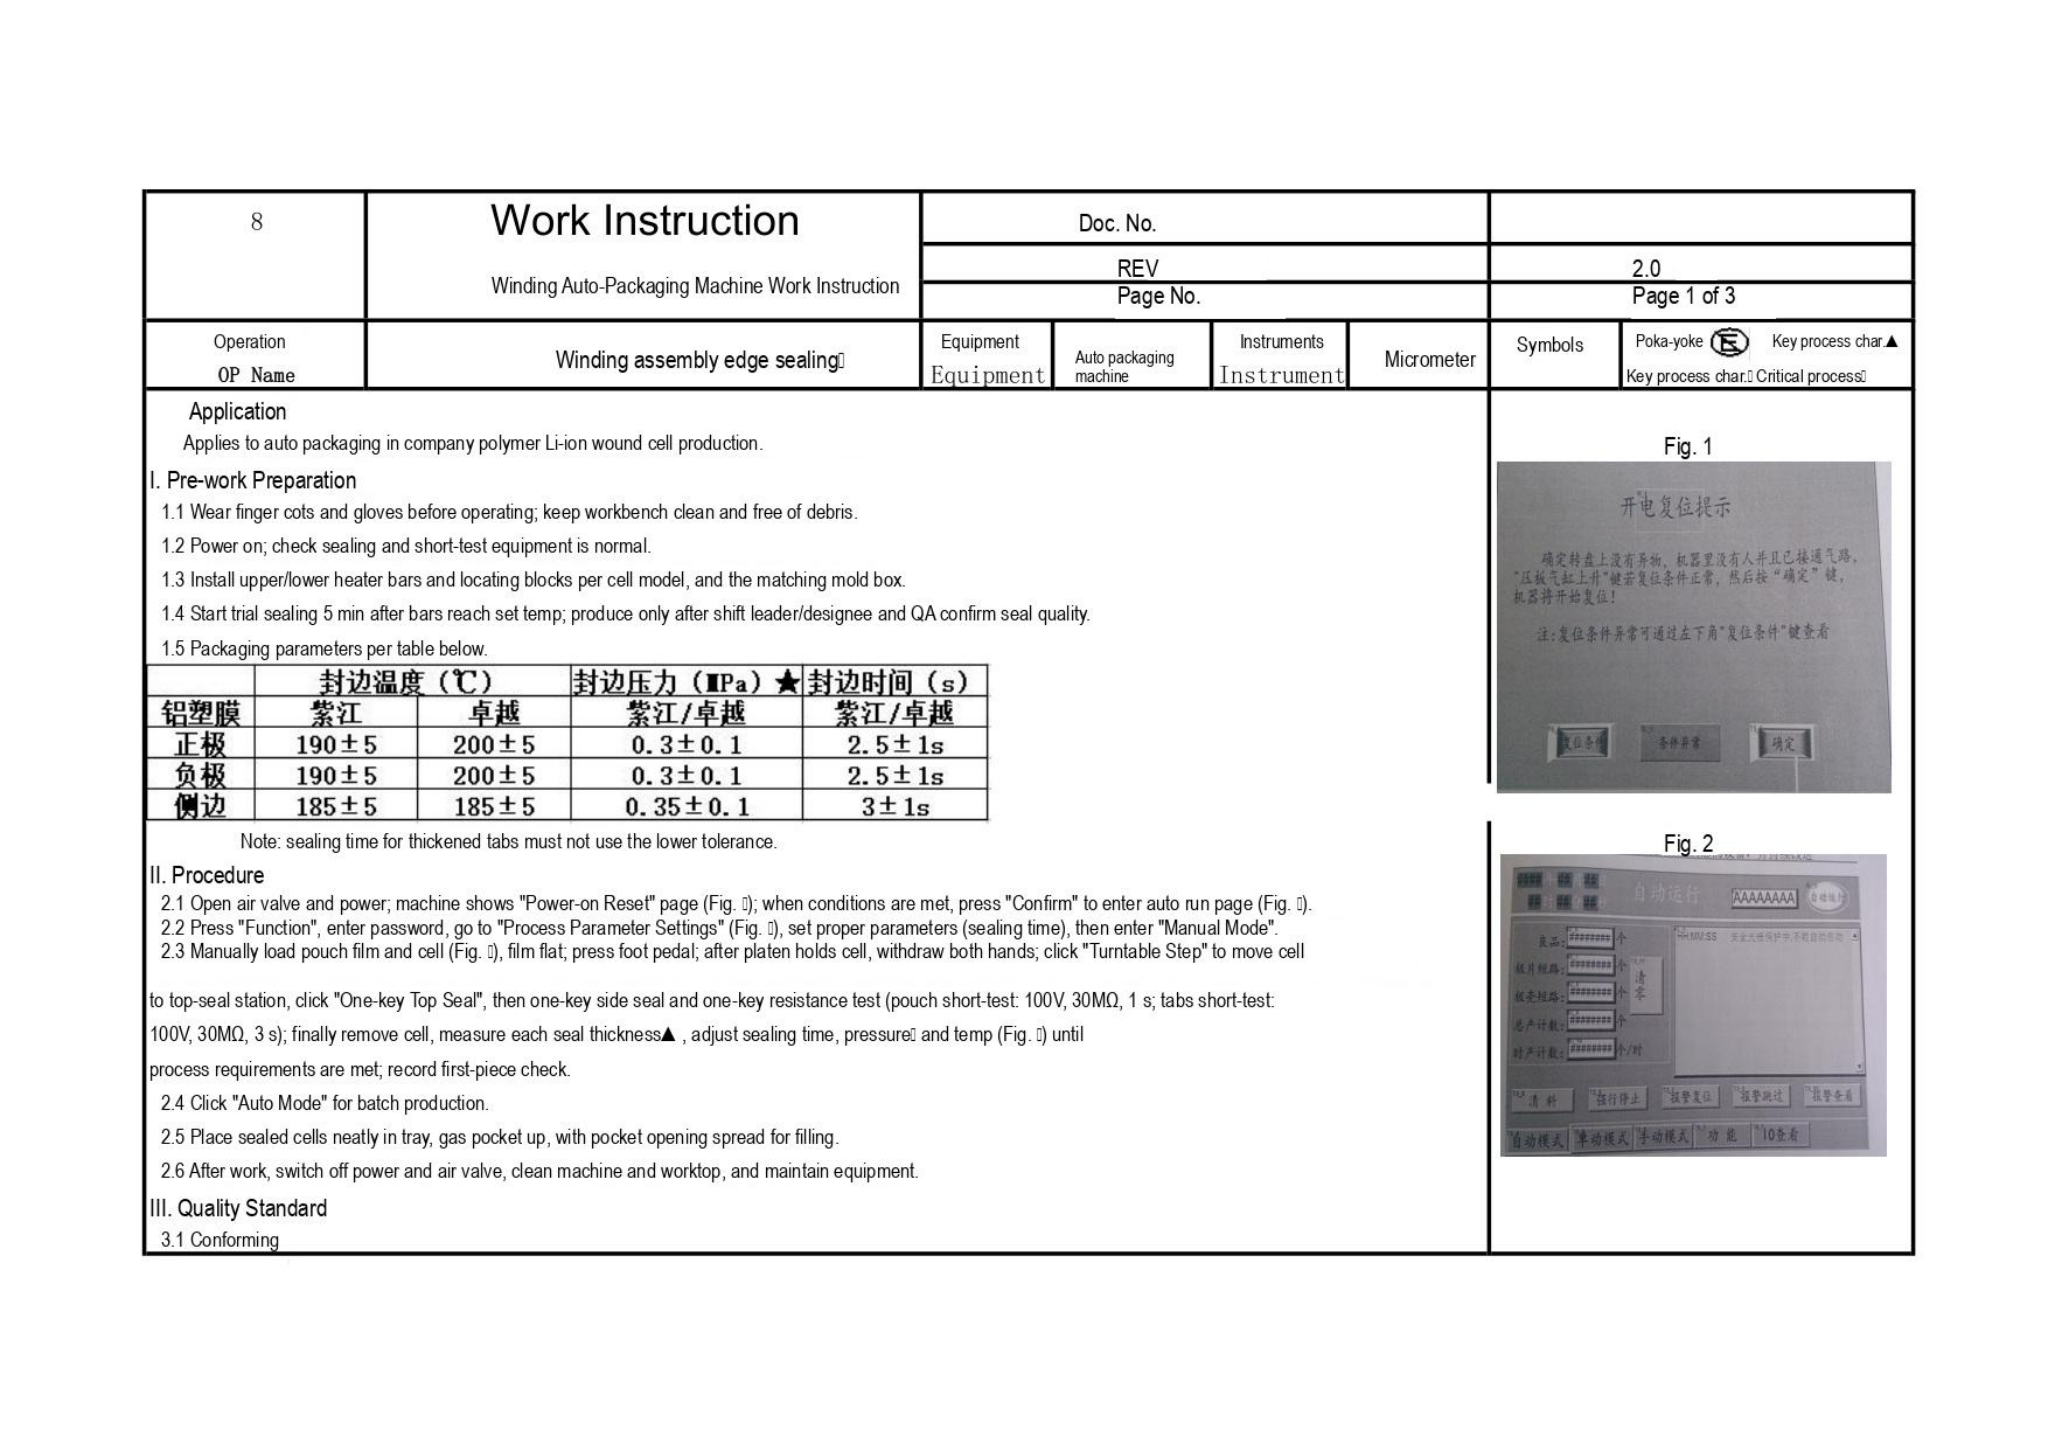8

# Work Instruction

Winding Auto-Packaging Machine Work Instruction

| Doc. No. | |
|---|---|
| REV | 2.0 |
| Page No. | Page 1 of 3 |

| Operation<br>OP Name | Winding assembly edge sealing | Equipment<br>Equipment | Auto packaging machine | Instruments<br>Instrument | Micrometer | Symbols | Poka-yoke Key process char.▲<br>Key process char. Critical process |
|---|---|---|---|---|---|---|---|

Application

Applies to auto packaging in company polymer Li-ion wound cell production.

I. Pre-work Preparation

1.1 Wear finger cots and gloves before operating; keep workbench clean and free of debris.

1.2 Power on; check sealing and short-test equipment is normal.

1.3 Install upper/lower heater bars and locating blocks per cell model, and the matching mold box.

1.4 Start trial sealing 5 min after bars reach set temp; produce only after shift leader/designee and QA confirm seal quality.

1.5 Packaging parameters per table below.

| | 封边温度（℃） | | 封边压力（MPa）★ | 封边时间（s） |
|---|---|---|---|---|
| 铝塑膜 | 紫江 | 卓越 | 紫江/卓越 | 紫江/卓越 |
| 正极 | 190±5 | 200±5 | 0.3±0.1 | 2.5±1s |
| 负极 | 190±5 | 200±5 | 0.3±0.1 | 2.5±1s |
| 侧边 | 185±5 | 185±5 | 0.35±0.1 | 3±1s |

Note: sealing time for thickened tabs must not use the lower tolerance.

II. Procedure

2.1 Open air valve and power; machine shows "Power-on Reset" page (Fig. ); when conditions are met, press "Confirm" to enter auto run page (Fig. ).

2.2 Press "Function", enter password, go to "Process Parameter Settings" (Fig. ), set proper parameters (sealing time), then enter "Manual Mode".

2.3 Manually load pouch film and cell (Fig. ), film flat; press foot pedal; after platen holds cell, withdraw both hands; click "Turntable Step" to move cell

to top-seal station, click "One-key Top Seal", then one-key side seal and one-key resistance test (pouch short-test: 100V, 30MΩ, 1 s; tabs short-test: 100V, 30MΩ, 3 s); finally remove cell, measure each seal thickness▲ , adjust sealing time, pressure and temp (Fig. ) until

process requirements are met; record first-piece check.

2.4 Click "Auto Mode" for batch production.

2.5 Place sealed cells neatly in tray, gas pocket up, with pocket opening spread for filling.

2.6 After work, switch off power and air valve, clean machine and worktop, and maintain equipment.

III. Quality Standard

3.1 Conforming

Fig. 1

开电复位提示

确定转盘上没有异物，机器里没有人并且已接通气路，"压板气缸上升"键若复位条件正常，然后按"确定"键，机器将开始复位！

注：复位条件异常可通过左下角"复位条件"键查看

复位条件 条件异常 确定

Fig. 2

自动运行 AAAAAAAA

良品 个

总产计数 个

时产计数 个/时

清零

HH:MM:SS

清 料 运行停止 报警复位 报警跳过 报警查看

自动模式 单动模式 手动模式 功 能 IO查看
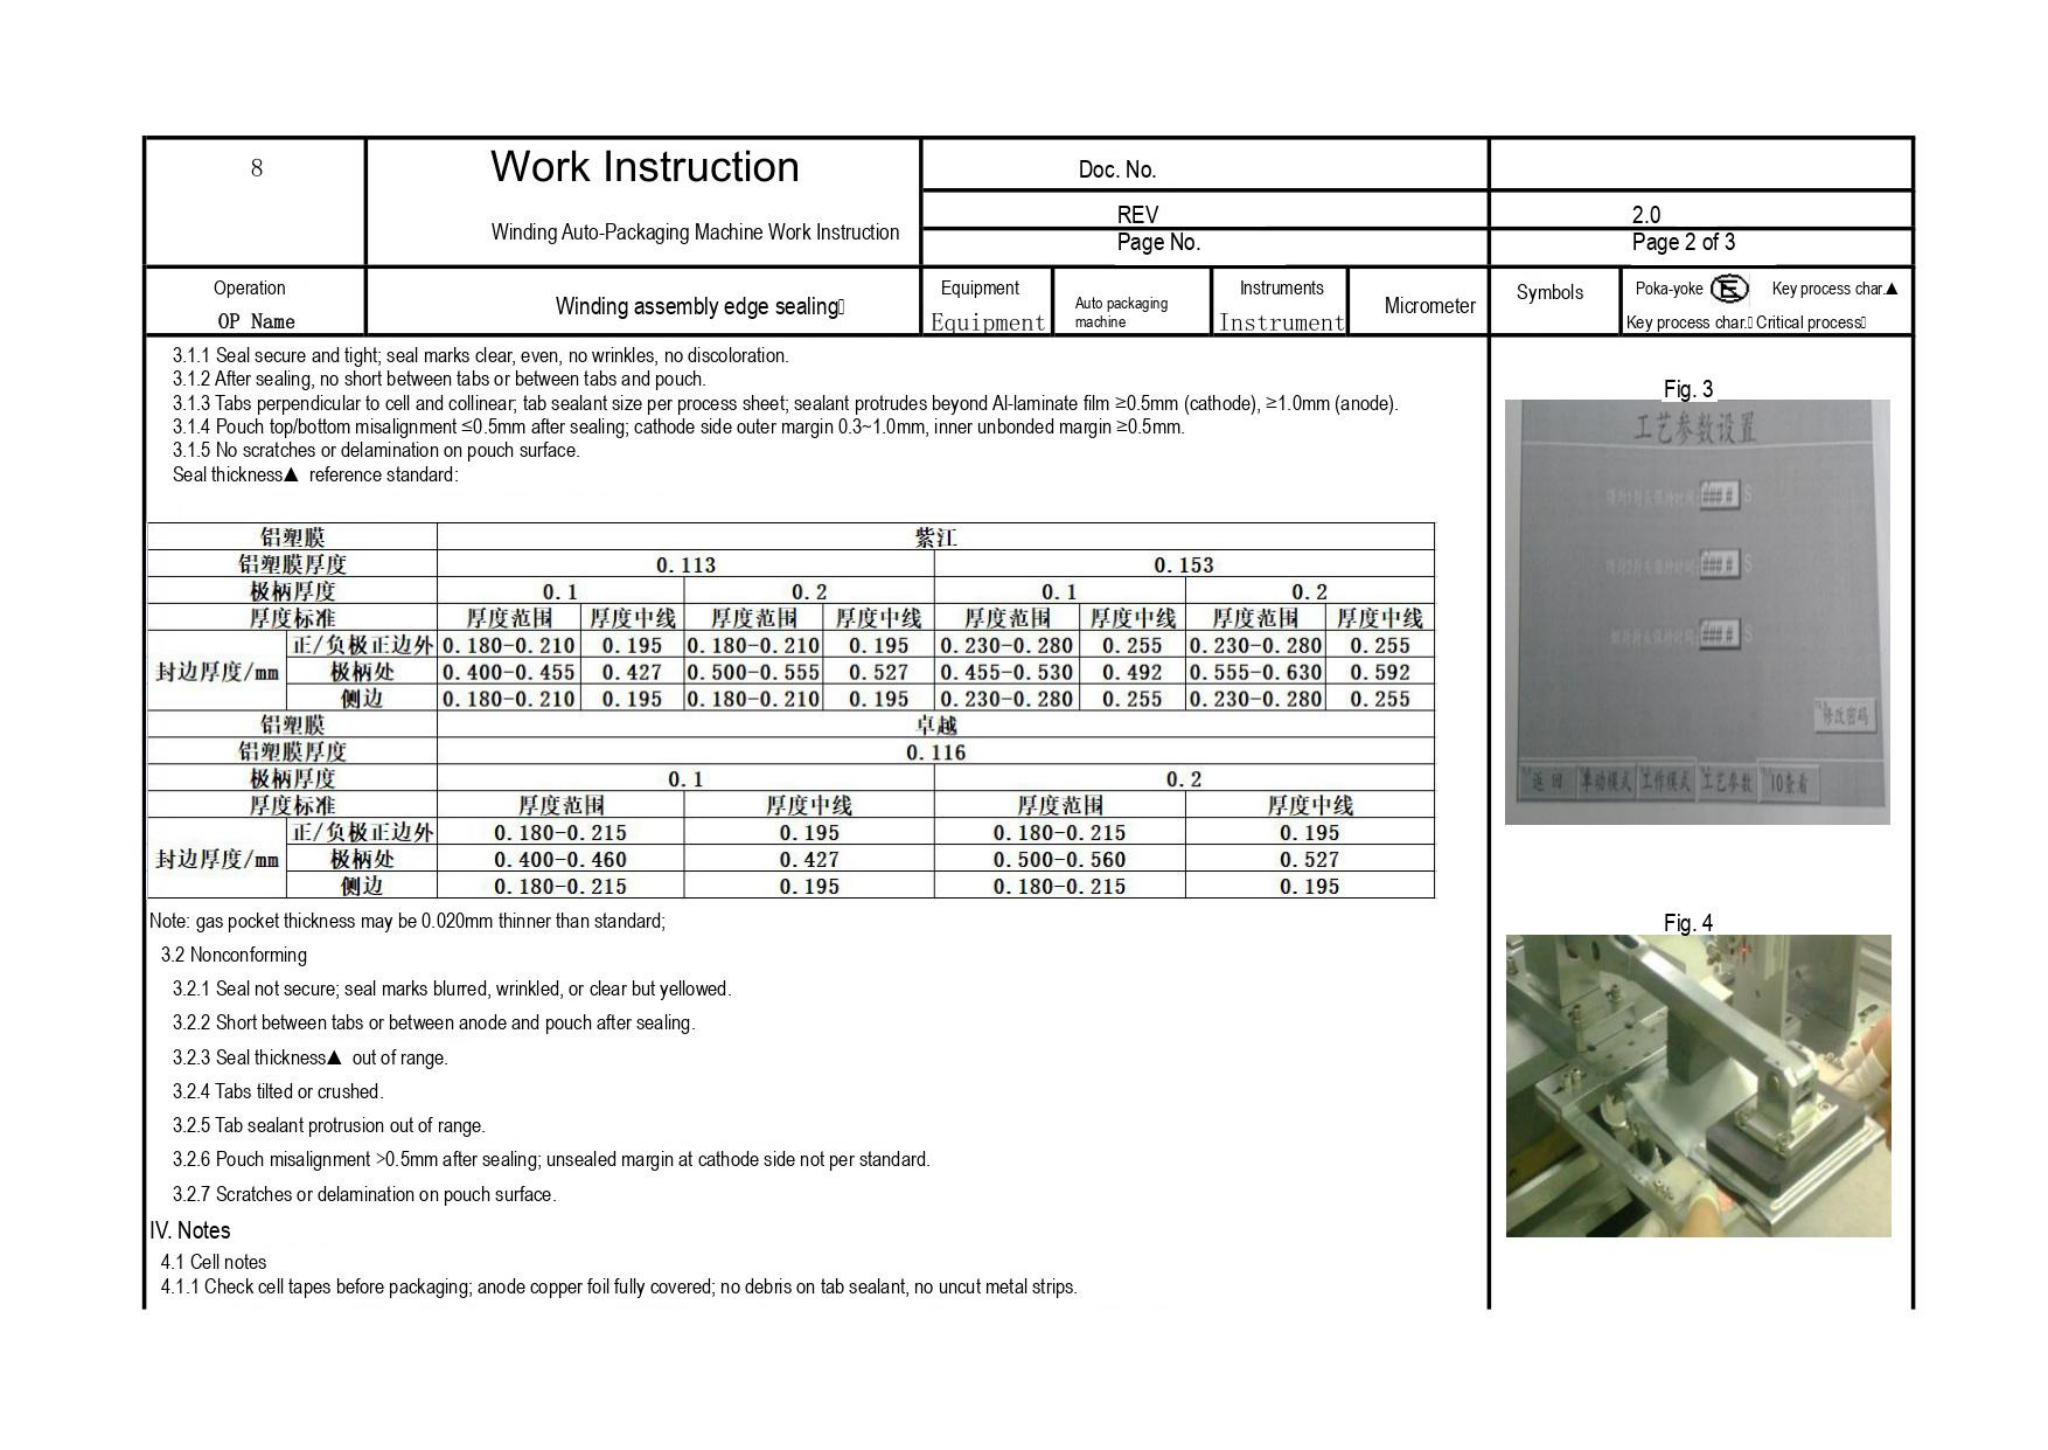| 8 | Work Instruction<br>Winding Auto-Packaging Machine Work Instruction | Doc. No. | |
|---|---|---|---|
| | | REV | 2.0 |
| | | Page No. | Page 2 of 3 |

| Operation<br>OP Name | Winding assembly edge sealing | Equipment<br>Equipment | Auto packaging machine | Instruments<br>Instrument | Micrometer | Symbols | Poka-yoke Key process char.▲<br>Key process char. Critical process |
|---|---|---|---|---|---|---|---|

3.1.1 Seal secure and tight; seal marks clear, even, no wrinkles, no discoloration.
3.1.2 After sealing, no short between tabs or between tabs and pouch.
3.1.3 Tabs perpendicular to cell and collinear; tab sealant size per process sheet; sealant protrudes beyond Al-laminate film ≥0.5mm (cathode), ≥1.0mm (anode).
3.1.4 Pouch top/bottom misalignment ≤0.5mm after sealing; cathode side outer margin 0.3~1.0mm, inner unbonded margin ≥0.5mm.
3.1.5 No scratches or delamination on pouch surface.
Seal thickness▲ reference standard:

| 铝塑膜 | | 紫江 | | | | | | | |
|---|---|---|---|---|---|---|---|---|---|
| 铝塑膜厚度 | | 0.113 | | | | 0.153 | | | |
| 极柄厚度 | | 0.1 | | 0.2 | | 0.1 | | 0.2 | |
| 厚度标准 | | 厚度范围 | 厚度中线 | 厚度范围 | 厚度中线 | 厚度范围 | 厚度中线 | 厚度范围 | 厚度中线 |
| 封边厚度/mm | 正/负极正边外 | 0.180-0.210 | 0.195 | 0.180-0.210 | 0.195 | 0.230-0.280 | 0.255 | 0.230-0.280 | 0.255 |
| 封边厚度/mm | 极柄处 | 0.400-0.455 | 0.427 | 0.500-0.555 | 0.527 | 0.455-0.530 | 0.492 | 0.555-0.630 | 0.592 |
| 封边厚度/mm | 侧边 | 0.180-0.210 | 0.195 | 0.180-0.210 | 0.195 | 0.230-0.280 | 0.255 | 0.230-0.280 | 0.255 |

| 铝塑膜 | | 卓越 | | | |
|---|---|---|---|---|---|
| 铝塑膜厚度 | | 0.116 | | | |
| 极柄厚度 | | 0.1 | | 0.2 | |
| 厚度标准 | | 厚度范围 | 厚度中线 | 厚度范围 | 厚度中线 |
| 封边厚度/mm | 正/负极正边外 | 0.180-0.215 | 0.195 | 0.180-0.215 | 0.195 |
| 封边厚度/mm | 极柄处 | 0.400-0.460 | 0.427 | 0.500-0.560 | 0.527 |
| 封边厚度/mm | 侧边 | 0.180-0.215 | 0.195 | 0.180-0.215 | 0.195 |

Note: gas pocket thickness may be 0.020mm thinner than standard;

3.2 Nonconforming
3.2.1 Seal not secure; seal marks blurred, wrinkled, or clear but yellowed.
3.2.2 Short between tabs or between anode and pouch after sealing.
3.2.3 Seal thickness▲ out of range.
3.2.4 Tabs tilted or crushed.
3.2.5 Tab sealant protrusion out of range.
3.2.6 Pouch misalignment >0.5mm after sealing; unsealed margin at cathode side not per standard.
3.2.7 Scratches or delamination on pouch surface.

IV. Notes
4.1 Cell notes
4.1.1 Check cell tapes before packaging; anode copper foil fully covered; no debris on tab sealant, no uncut metal strips.

Fig. 3
工艺参数设置
修改密码
返回 手动模式 工作模式 工艺参数 IO查看

Fig. 4
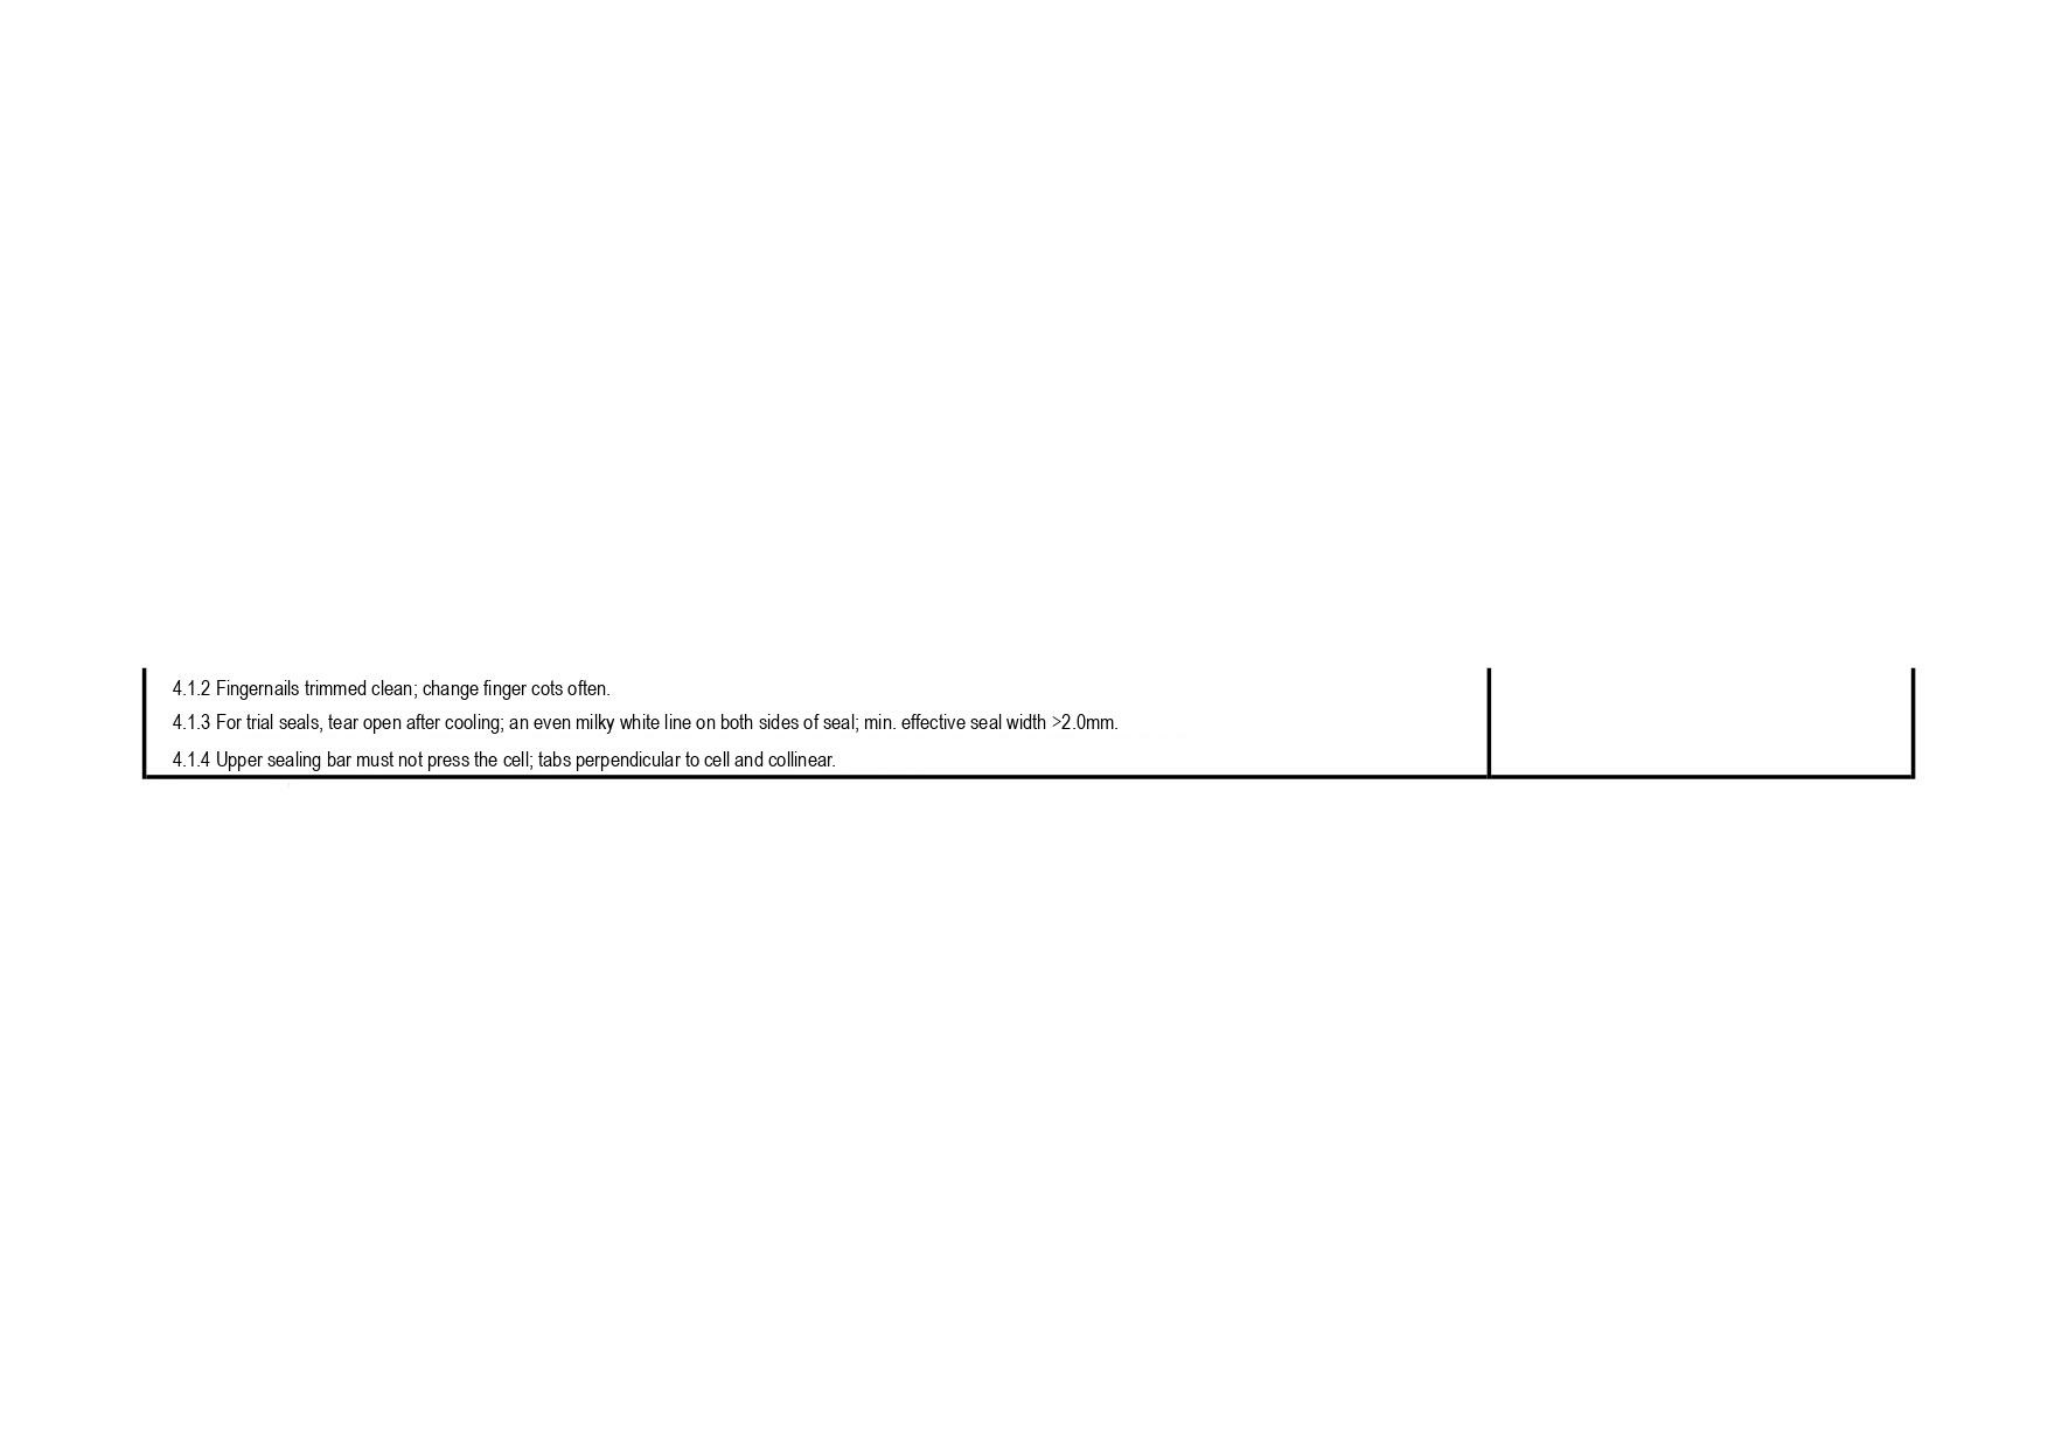| | |
|---|---|
| 4.1.2 Fingernails trimmed clean; change finger cots often.<br>4.1.3 For trial seals, tear open after cooling; an even milky white line on both sides of seal; min. effective seal width >2.0mm.<br>4.1.4 Upper sealing bar must not press the cell; tabs perpendicular to cell and collinear. | |
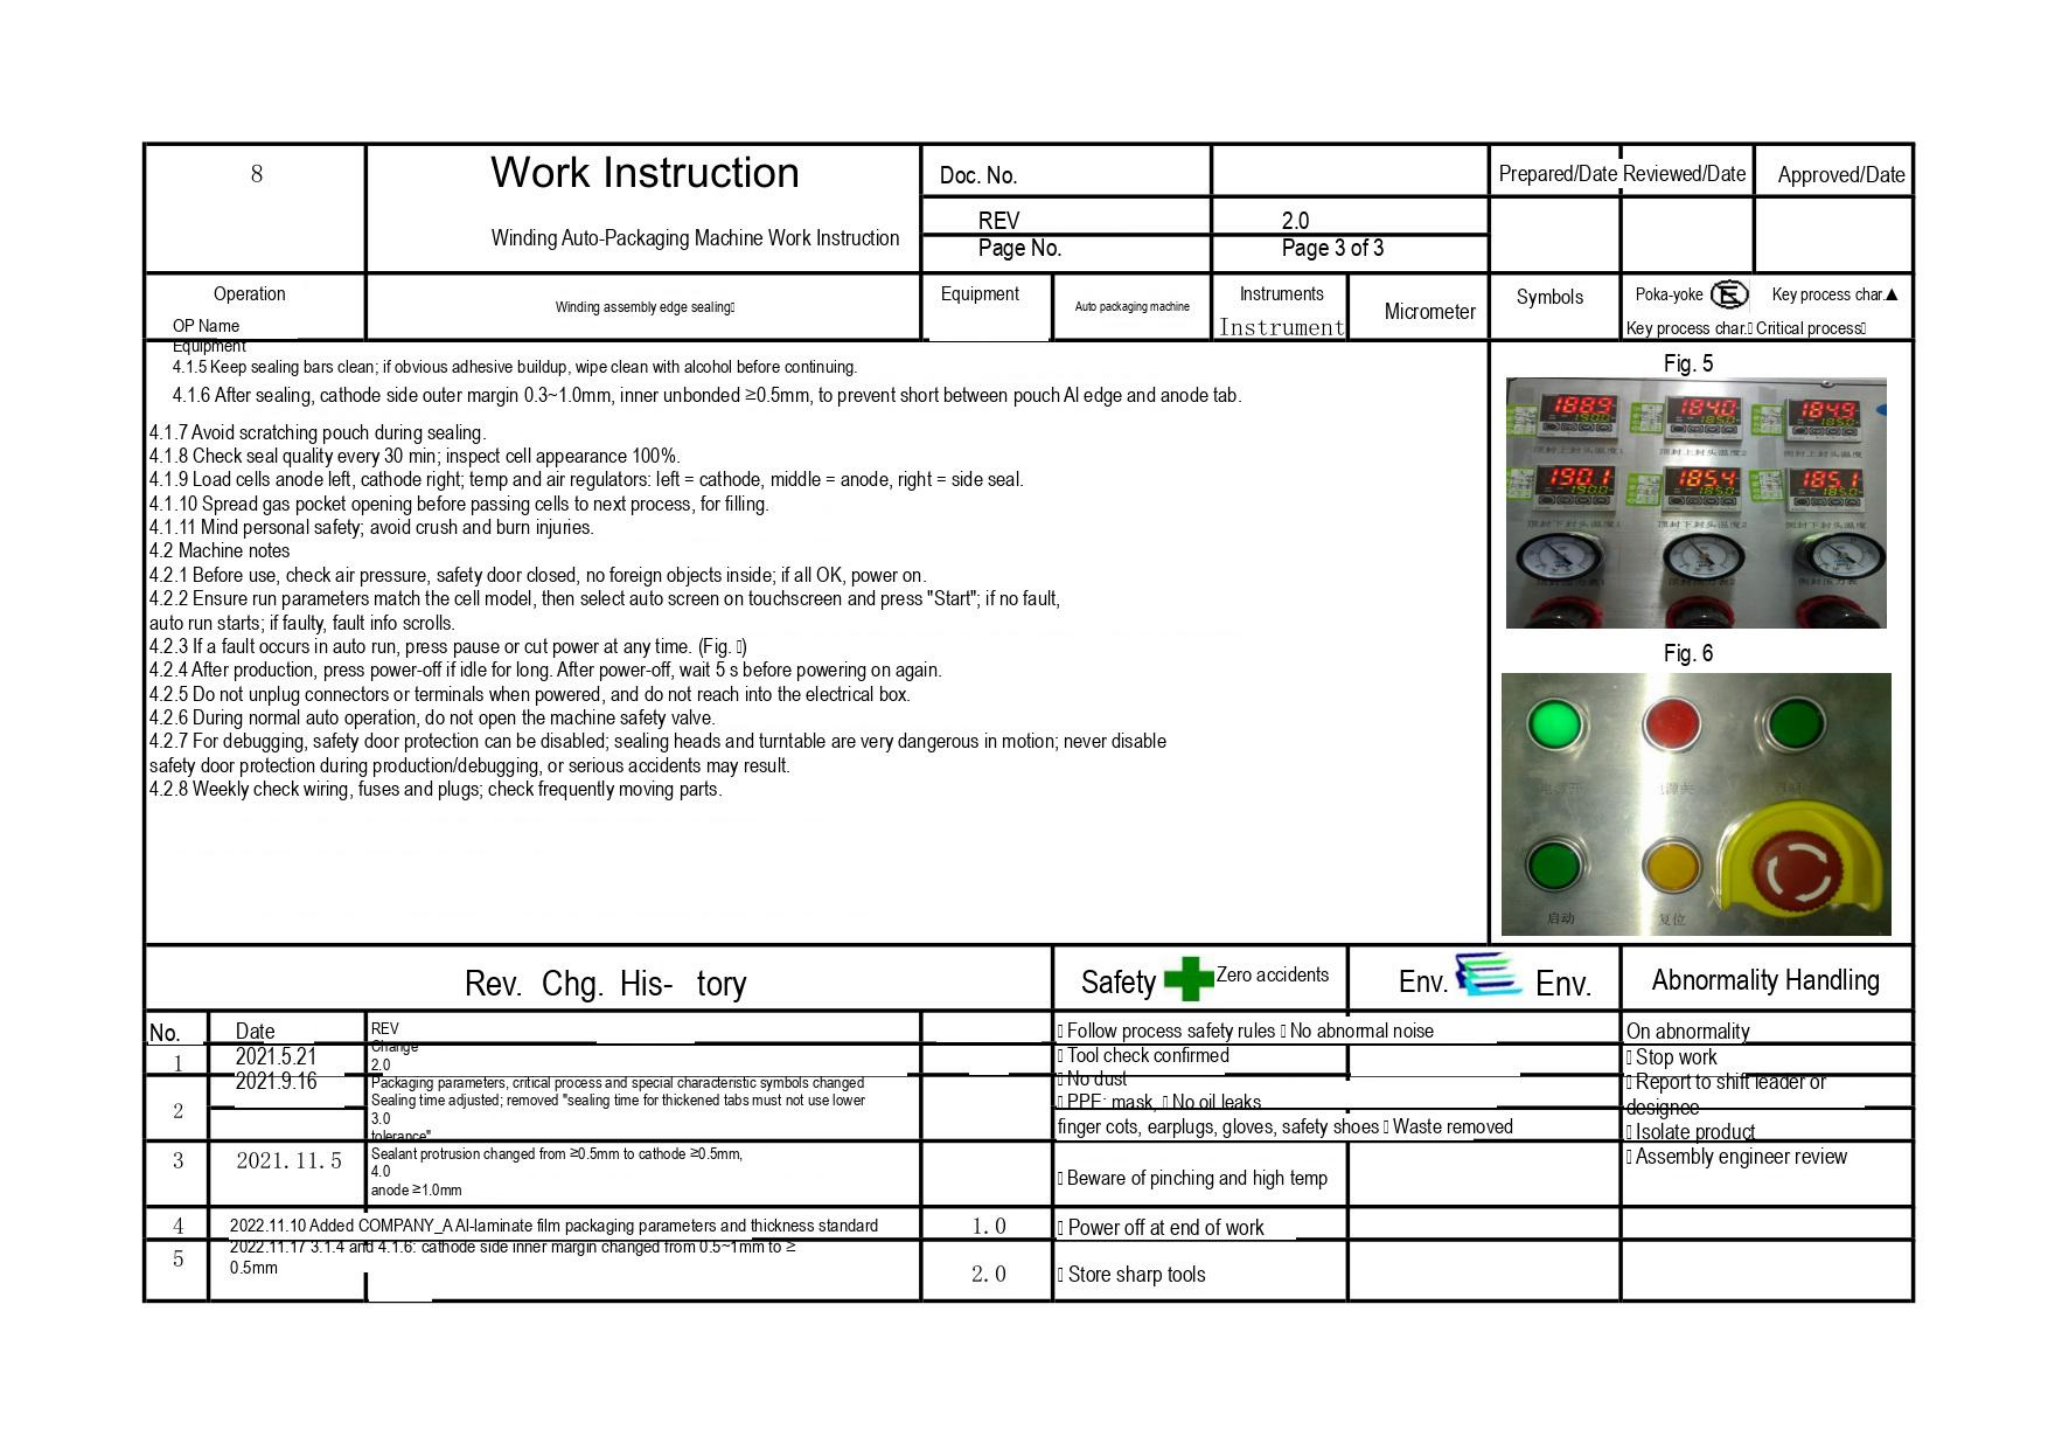| 8 | Work Instruction<br>Winding Auto-Packaging Machine Work Instruction | Doc. No. | | Prepared/Date | Reviewed/Date | Approved/Date |
|---|---|---|---|---|---|---|
| | | REV | 2.0 | | | |
| | | Page No. | Page 3 of 3 | | | |

| Operation<br>OP Name | Winding assembly edge sealing | Equipment | Auto packaging machine | Instruments<br>Instrument | Micrometer | Symbols | Poka-yoke Key process char.▲<br>Key process char. Critical process |
|---|---|---|---|---|---|---|---|

Equipment
4.1.5 Keep sealing bars clean; if obvious adhesive buildup, wipe clean with alcohol before continuing.
4.1.6 After sealing, cathode side outer margin 0.3~1.0mm, inner unbonded ≥0.5mm, to prevent short between pouch Al edge and anode tab.
4.1.7 Avoid scratching pouch during sealing.
4.1.8 Check seal quality every 30 min; inspect cell appearance 100%.
4.1.9 Load cells anode left, cathode right; temp and air regulators: left = cathode, middle = anode, right = side seal.
4.1.10 Spread gas pocket opening before passing cells to next process, for filling.
4.1.11 Mind personal safety; avoid crush and burn injuries.
4.2 Machine notes
4.2.1 Before use, check air pressure, safety door closed, no foreign objects inside; if all OK, power on.
4.2.2 Ensure run parameters match the cell model, then select auto screen on touchscreen and press "Start"; if no fault, auto run starts; if faulty, fault info scrolls.
4.2.3 If a fault occurs in auto run, press pause or cut power at any time. (Fig. )
4.2.4 After production, press power-off if idle for long. After power-off, wait 5 s before powering on again.
4.2.5 Do not unplug connectors or terminals when powered, and do not reach into the electrical box.
4.2.6 During normal auto operation, do not open the machine safety valve.
4.2.7 For debugging, safety door protection can be disabled; sealing heads and turntable are very dangerous in motion; never disable safety door protection during production/debugging, or serious accidents may result.
4.2.8 Weekly check wiring, fuses and plugs; check frequently moving parts.

Fig. 5
188.9 184.0 184.9
190.1 185.4 185.1
1900 1850 1850

Fig. 6
启动 复位

| Rev. Chg. His- tory | | | | Safety Zero accidents | Env. Env. | Abnormality Handling |
|---|---|---|---|---|---|---|
| No. | Date | REV Change | | Follow process safety rules No abnormal noise | | On abnormality |
| 1 | 2021.5.21 | 2.0 | | Tool check confirmed | | Stop work |
| 2 | 2021.9.16 | Packaging parameters, critical process and special characteristic symbols changed<br>Sealing time adjusted; removed "sealing time for thickened tabs must not use lower tolerance"<br>3.0 | | No dust<br>PPE: mask, finger cots, earplugs, gloves, safety shoes | No oil leaks<br>Waste removed | Report to shift leader or designee<br>Isolate product |
| 3 | 2021. 11. 5 | Sealant protrusion changed from ≥0.5mm to cathode ≥0.5mm, anode ≥1.0mm<br>4.0 | | Beware of pinching and high temp | | Assembly engineer review |
| 4 | 2022.11.10 Added COMPANY_A Al-laminate film packaging parameters and thickness standard | | 1. 0 | Power off at end of work | | |
| 5 | 2022.11.17 3.1.4 and 4.1.6: cathode side inner margin changed from 0.5~1mm to ≥ 0.5mm | | 2. 0 | Store sharp tools | | |